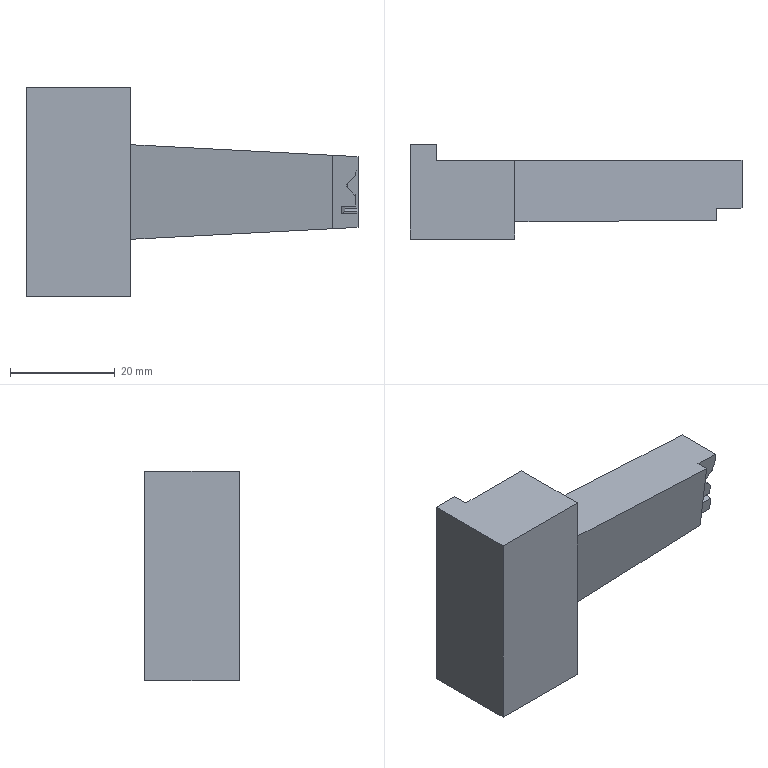Part | STEP file | 1 solid | 33 faces | box 63.268 x 18 x 40 mm | volume 19584 mm3 | plane 27 | cylinder 6 | commonest cylinder face diameters 0.603 x4 1.005 x2